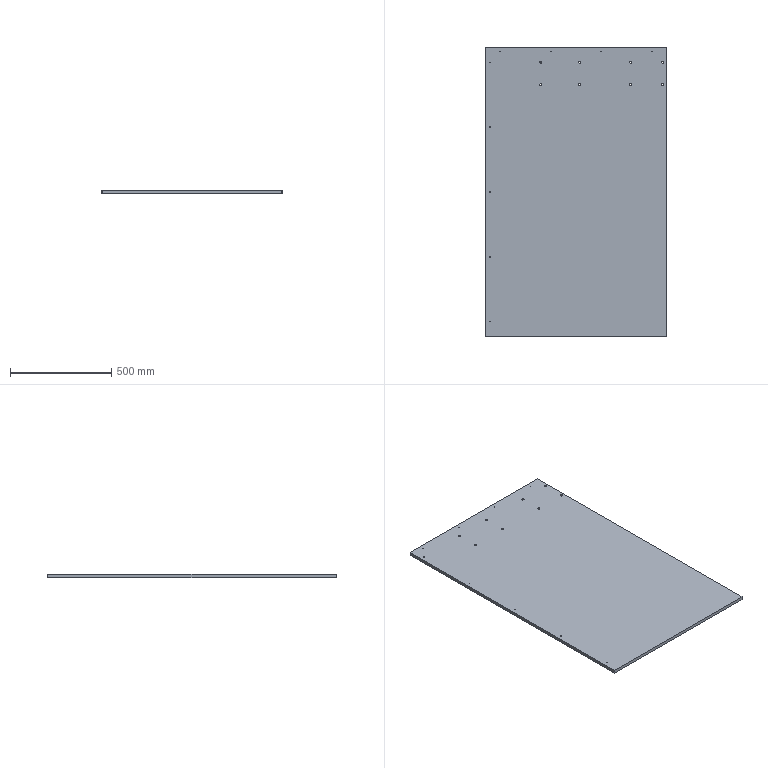Part | NX | features BREP 1 | 1 solid | 44 faces | box 895 x 1433 x 16 mm | volume 20507957 mm3 | cylinder 34 | plane 10 | commonest cylinder face diameters 3.3 x18 10.5 x16
STEP:
#1=CARTESIAN_POINT('',(-168.75,531.5,16.));
#2=VERTEX_POINT('',#1);
#3=CARTESIAN_POINT('',(-179.25,531.5,16.));
#4=VERTEX_POINT('',#3);
#5=CARTESIAN_POINT('',(-174.,531.5,16.));
#6=DIRECTION('',(0.,0.,-1.));
#7=DIRECTION('',(-1.,0.,0.));
#8=AXIS2_PLACEMENT_3D('',#5,#6,#7);
#9=CIRCLE('',#8,5.25);
#10=EDGE_CURVE('',#2,#4,#9,.T.);
#11=ORIENTED_EDGE('',*,*,#10,.F.);
#12=CARTESIAN_POINT('',(-168.75,531.5,0.));
#13=VERTEX_POINT('',#12);
#14=CARTESIAN_POINT('',(-168.75,531.5,0.));
#15=DIRECTION('',(0.,0.,-1.));
#16=VECTOR('',#15,1000.);
#17=LINE('',#14,#16);
#18=EDGE_CURVE('',#2,#13,#17,.T.);
#19=ORIENTED_EDGE('',*,*,#18,.T.);
#20=CARTESIAN_POINT('',(-179.25,531.5,0.));
#21=VERTEX_POINT('',#20);
#22=CARTESIAN_POINT('',(-174.,531.5,0.));
#23=DIRECTION('',(0.,0.,-1.));
#24=DIRECTION('',(-1.,0.,0.));
#25=AXIS2_PLACEMENT_3D('',#22,#23,#24);
#26=CIRCLE('',#25,5.25);
#27=EDGE_CURVE('',#13,#21,#26,.T.);
#28=ORIENTED_EDGE('',*,*,#27,.T.);
#29=CARTESIAN_POINT('',(-179.25,531.5,0.));
#30=DIRECTION('',(0.,0.,-1.));
#31=VECTOR('',#30,1000.);
#32=LINE('',#29,#31);
#33=EDGE_CURVE('',#4,#21,#32,.T.);
#34=ORIENTED_EDGE('',*,*,#33,.F.);
#35=EDGE_LOOP('',(#11,#19,#28,#34));
#36=FACE_BOUND('',#35,.T.);
#37=CARTESIAN_POINT('',(-174.,531.5,0.));
#38=DIRECTION('',(0.,0.,-1.));
#39=DIRECTION('',(-1.,0.,0.));
#40=AXIS2_PLACEMENT_3D('',#37,#38,#39);
#41=CYLINDRICAL_SURFACE('',#40,5.25);
#42=ADVANCED_FACE('',(#36),#41,.F.);
#43=CARTESIAN_POINT('',(-168.75,641.5,16.));
#44=VERTEX_POINT('',#43);
#45=CARTESIAN_POINT('',(-179.25,641.5,16.));
#46=VERTEX_POINT('',#45);
#47=CARTESIAN_POINT('',(-174.,641.5,16.));
#48=DIRECTION('',(0.,0.,-1.));
#49=DIRECTION('',(-1.,0.,0.));
#50=AXIS2_PLACEMENT_3D('',#47,#48,#49);
#51=CIRCLE('',#50,5.25);
#52=EDGE_CURVE('',#44,#46,#51,.T.);
#53=ORIENTED_EDGE('',*,*,#52,.F.);
#54=CARTESIAN_POINT('',(-168.75,641.5,0.));
#55=VERTEX_POINT('',#54);
#56=CARTESIAN_POINT('',(-168.75,641.5,0.));
#57=DIRECTION('',(0.,0.,-1.));
#58=VECTOR('',#57,1000.);
#59=LINE('',#56,#58);
#60=EDGE_CURVE('',#44,#55,#59,.T.);
#61=ORIENTED_EDGE('',*,*,#60,.T.);
#62=CARTESIAN_POINT('',(-179.25,641.5,0.));
#63=VERTEX_POINT('',#62);
#64=CARTESIAN_POINT('',(-174.,641.5,0.));
#65=DIRECTION('',(0.,0.,-1.));
#66=DIRECTION('',(-1.,0.,0.));
#67=AXIS2_PLACEMENT_3D('',#64,#65,#66);
#68=CIRCLE('',#67,5.25);
#69=EDGE_CURVE('',#55,#63,#68,.T.);
#70=ORIENTED_EDGE('',*,*,#69,.T.);
#71=CARTESIAN_POINT('',(-179.25,641.5,0.));
#72=DIRECTION('',(0.,0.,-1.));
#73=VECTOR('',#72,1000.);
#74=LINE('',#71,#73);
#75=EDGE_CURVE('',#46,#63,#74,.T.);
#76=ORIENTED_EDGE('',*,*,#75,.F.);
#77=EDGE_LOOP('',(#53,#61,#70,#76));
#78=FACE_BOUND('',#77,.T.);
#79=CARTESIAN_POINT('',(-174.,641.5,0.));
#80=DIRECTION('',(0.,0.,-1.));
#81=DIRECTION('',(-1.,0.,0.));
#82=AXIS2_PLACEMENT_3D('',#79,#80,#81);
#83=CYLINDRICAL_SURFACE('',#82,5.25);
#84=ADVANCED_FACE('',(#78),#83,.F.);
#85=CARTESIAN_POINT('',(23.75,531.5,16.));
#86=VERTEX_POINT('',#85);
#87=CARTESIAN_POINT('',(13.25,531.5,16.));
#88=VERTEX_POINT('',#87);
#89=CARTESIAN_POINT('',(18.5,531.5,16.));
#90=DIRECTION('',(0.,0.,-1.));
#91=DIRECTION('',(-1.,0.,0.));
#92=AXIS2_PLACEMENT_3D('',#89,#90,#91);
#93=CIRCLE('',#92,5.25);
#94=EDGE_CURVE('',#86,#88,#93,.T.);
#95=ORIENTED_EDGE('',*,*,#94,.F.);
#96=CARTESIAN_POINT('',(23.75,531.5,0.));
#97=VERTEX_POINT('',#96);
#98=CARTESIAN_POINT('',(23.75,531.5,0.));
#99=DIRECTION('',(0.,0.,-1.));
#100=VECTOR('',#99,1000.);
#101=LINE('',#98,#100);
#102=EDGE_CURVE('',#86,#97,#101,.T.);
#103=ORIENTED_EDGE('',*,*,#102,.T.);
#104=CARTESIAN_POINT('',(13.25,531.5,0.));
#105=VERTEX_POINT('',#104);
#106=CARTESIAN_POINT('',(18.5,531.5,0.));
#107=DIRECTION('',(0.,0.,-1.));
#108=DIRECTION('',(-1.,0.,0.));
#109=AXIS2_PLACEMENT_3D('',#106,#107,#108);
#110=CIRCLE('',#109,5.25);
#111=EDGE_CURVE('',#97,#105,#110,.T.);
#112=ORIENTED_EDGE('',*,*,#111,.T.);
#113=CARTESIAN_POINT('',(13.25,531.5,0.));
#114=DIRECTION('',(0.,0.,-1.));
#115=VECTOR('',#114,1000.);
#116=LINE('',#113,#115);
#117=EDGE_CURVE('',#88,#105,#116,.T.);
#118=ORIENTED_EDGE('',*,*,#117,.F.);
#119=EDGE_LOOP('',(#95,#103,#112,#118));
#120=FACE_BOUND('',#119,.T.);
#121=CARTESIAN_POINT('',(18.5,531.5,0.));
#122=DIRECTION('',(0.,0.,-1.));
#123=DIRECTION('',(-1.,0.,0.));
#124=AXIS2_PLACEMENT_3D('',#121,#122,#123);
#125=CYLINDRICAL_SURFACE('',#124,5.25);
#126=ADVANCED_FACE('',(#120),#125,.F.);
#127=CARTESIAN_POINT('',(23.75,641.5,16.));
#128=VERTEX_POINT('',#127);
#129=CARTESIAN_POINT('',(13.25,641.5,16.));
#130=VERTEX_POINT('',#129);
#131=CARTESIAN_POINT('',(18.5,641.5,16.));
#132=DIRECTION('',(0.,0.,-1.));
#133=DIRECTION('',(-1.,0.,0.));
#134=AXIS2_PLACEMENT_3D('',#131,#132,#133);
#135=CIRCLE('',#134,5.25);
#136=EDGE_CURVE('',#128,#130,#135,.T.);
#137=ORIENTED_EDGE('',*,*,#136,.F.);
#138=CARTESIAN_POINT('',(23.75,641.5,0.));
#139=VERTEX_POINT('',#138);
#140=CARTESIAN_POINT('',(23.75,641.5,0.));
#141=DIRECTION('',(0.,0.,-1.));
#142=VECTOR('',#141,1000.);
#143=LINE('',#140,#142);
#144=EDGE_CURVE('',#128,#139,#143,.T.);
#145=ORIENTED_EDGE('',*,*,#144,.T.);
#146=CARTESIAN_POINT('',(13.25,641.5,0.));
#147=VERTEX_POINT('',#146);
#148=CARTESIAN_POINT('',(18.5,641.5,0.));
#149=DIRECTION('',(0.,0.,-1.));
#150=DIRECTION('',(-1.,0.,0.));
#151=AXIS2_PLACEMENT_3D('',#148,#149,#150);
#152=CIRCLE('',#151,5.25);
#153=EDGE_CURVE('',#139,#147,#152,.T.);
#154=ORIENTED_EDGE('',*,*,#153,.T.);
#155=CARTESIAN_POINT('',(13.25,641.5,0.));
#156=DIRECTION('',(0.,0.,-1.));
#157=VECTOR('',#156,1000.);
#158=LINE('',#155,#157);
#159=EDGE_CURVE('',#130,#147,#158,.T.);
#160=ORIENTED_EDGE('',*,*,#159,.F.);
#161=EDGE_LOOP('',(#137,#145,#154,#160));
#162=FACE_BOUND('',#161,.T.);
#163=CARTESIAN_POINT('',(18.5,641.5,0.));
#164=DIRECTION('',(0.,0.,-1.));
#165=DIRECTION('',(-1.,0.,0.));
#166=AXIS2_PLACEMENT_3D('',#163,#164,#165);
#167=CYLINDRICAL_SURFACE('',#166,5.25);
#168=ADVANCED_FACE('',(#162),#167,.F.);
#169=CARTESIAN_POINT('',(275.75,531.5,16.));
#170=VERTEX_POINT('',#169);
#171=CARTESIAN_POINT('',(265.25,531.5,16.));
#172=VERTEX_POINT('',#171);
#173=CARTESIAN_POINT('',(270.5,531.5,16.));
#174=DIRECTION('',(0.,0.,-1.));
#175=DIRECTION('',(-1.,0.,0.));
#176=AXIS2_PLACEMENT_3D('',#173,#174,#175);
#177=CIRCLE('',#176,5.25);
#178=EDGE_CURVE('',#170,#172,#177,.T.);
#179=ORIENTED_EDGE('',*,*,#178,.F.);
#180=CARTESIAN_POINT('',(275.75,531.5,0.));
#181=VERTEX_POINT('',#180);
#182=CARTESIAN_POINT('',(275.75,531.5,0.));
#183=DIRECTION('',(0.,0.,-1.));
#184=VECTOR('',#183,1000.);
#185=LINE('',#182,#184);
#186=EDGE_CURVE('',#170,#181,#185,.T.);
#187=ORIENTED_EDGE('',*,*,#186,.T.);
#188=CARTESIAN_POINT('',(265.25,531.5,0.));
#189=VERTEX_POINT('',#188);
#190=CARTESIAN_POINT('',(270.5,531.5,0.));
#191=DIRECTION('',(0.,0.,-1.));
#192=DIRECTION('',(-1.,0.,0.));
#193=AXIS2_PLACEMENT_3D('',#190,#191,#192);
#194=CIRCLE('',#193,5.25);
#195=EDGE_CURVE('',#181,#189,#194,.T.);
#196=ORIENTED_EDGE('',*,*,#195,.T.);
#197=CARTESIAN_POINT('',(265.25,531.5,0.));
#198=DIRECTION('',(0.,0.,-1.));
#199=VECTOR('',#198,1000.);
#200=LINE('',#197,#199);
#201=EDGE_CURVE('',#172,#189,#200,.T.);
#202=ORIENTED_EDGE('',*,*,#201,.F.);
#203=EDGE_LOOP('',(#179,#187,#196,#202));
#204=FACE_BOUND('',#203,.T.);
#205=CARTESIAN_POINT('',(270.5,531.5,0.));
#206=DIRECTION('',(0.,0.,-1.));
#207=DIRECTION('',(-1.,0.,0.));
#208=AXIS2_PLACEMENT_3D('',#205,#206,#207);
#209=CYLINDRICAL_SURFACE('',#208,5.25);
#210=ADVANCED_FACE('',(#204),#209,.F.);
#211=CARTESIAN_POINT('',(275.75,641.5,16.));
#212=VERTEX_POINT('',#211);
#213=CARTESIAN_POINT('',(265.25,641.5,16.));
#214=VERTEX_POINT('',#213);
#215=CARTESIAN_POINT('',(270.5,641.5,16.));
#216=DIRECTION('',(0.,0.,-1.));
#217=DIRECTION('',(-1.,0.,0.));
#218=AXIS2_PLACEMENT_3D('',#215,#216,#217);
#219=CIRCLE('',#218,5.25);
#220=EDGE_CURVE('',#212,#214,#219,.T.);
#221=ORIENTED_EDGE('',*,*,#220,.F.);
#222=CARTESIAN_POINT('',(275.75,641.5,0.));
#223=VERTEX_POINT('',#222);
#224=CARTESIAN_POINT('',(275.75,641.5,0.));
#225=DIRECTION('',(0.,0.,-1.));
#226=VECTOR('',#225,1000.);
#227=LINE('',#224,#226);
#228=EDGE_CURVE('',#212,#223,#227,.T.);
#229=ORIENTED_EDGE('',*,*,#228,.T.);
#230=CARTESIAN_POINT('',(265.25,641.5,0.));
#231=VERTEX_POINT('',#230);
#232=CARTESIAN_POINT('',(270.5,641.5,0.));
#233=DIRECTION('',(0.,0.,-1.));
#234=DIRECTION('',(-1.,0.,0.));
#235=AXIS2_PLACEMENT_3D('',#232,#233,#234);
#236=CIRCLE('',#235,5.25);
#237=EDGE_CURVE('',#223,#231,#236,.T.);
#238=ORIENTED_EDGE('',*,*,#237,.T.);
#239=CARTESIAN_POINT('',(265.25,641.5,0.));
#240=DIRECTION('',(0.,0.,-1.));
#241=VECTOR('',#240,1000.);
#242=LINE('',#239,#241);
#243=EDGE_CURVE('',#214,#231,#242,.T.);
#244=ORIENTED_EDGE('',*,*,#243,.F.);
#245=EDGE_LOOP('',(#221,#229,#238,#244));
#246=FACE_BOUND('',#245,.T.);
#247=CARTESIAN_POINT('',(270.5,641.5,0.));
#248=DIRECTION('',(0.,0.,-1.));
#249=DIRECTION('',(-1.,0.,0.));
#250=AXIS2_PLACEMENT_3D('',#247,#248,#249);
#251=CYLINDRICAL_SURFACE('',#250,5.25);
#252=ADVANCED_FACE('',(#246),#251,.F.);
#253=CARTESIAN_POINT('',(434.25,641.5,16.));
#254=VERTEX_POINT('',#253);
#255=CARTESIAN_POINT('',(423.75,641.5,16.));
#256=VERTEX_POINT('',#255);
#257=CARTESIAN_POINT('',(429.,641.5,16.));
#258=DIRECTION('',(0.,0.,-1.));
#259=DIRECTION('',(-1.,0.,0.));
#260=AXIS2_PLACEMENT_3D('',#257,#258,#259);
#261=CIRCLE('',#260,5.25);
#262=EDGE_CURVE('',#254,#256,#261,.T.);
#263=ORIENTED_EDGE('',*,*,#262,.F.);
#264=CARTESIAN_POINT('',(434.25,641.5,0.));
#265=VERTEX_POINT('',#264);
#266=CARTESIAN_POINT('',(434.25,641.5,0.));
#267=DIRECTION('',(0.,0.,-1.));
#268=VECTOR('',#267,1000.);
#269=LINE('',#266,#268);
#270=EDGE_CURVE('',#254,#265,#269,.T.);
#271=ORIENTED_EDGE('',*,*,#270,.T.);
#272=CARTESIAN_POINT('',(423.75,641.5,0.));
#273=VERTEX_POINT('',#272);
#274=CARTESIAN_POINT('',(429.,641.5,0.));
#275=DIRECTION('',(0.,0.,-1.));
#276=DIRECTION('',(-1.,0.,0.));
#277=AXIS2_PLACEMENT_3D('',#274,#275,#276);
#278=CIRCLE('',#277,5.25);
#279=EDGE_CURVE('',#265,#273,#278,.T.);
#280=ORIENTED_EDGE('',*,*,#279,.T.);
#281=CARTESIAN_POINT('',(423.75,641.5,0.));
#282=DIRECTION('',(0.,0.,-1.));
#283=VECTOR('',#282,1000.);
#284=LINE('',#281,#283);
#285=EDGE_CURVE('',#256,#273,#284,.T.);
#286=ORIENTED_EDGE('',*,*,#285,.F.);
#287=EDGE_LOOP('',(#263,#271,#280,#286));
#288=FACE_BOUND('',#287,.T.);
#289=CARTESIAN_POINT('',(429.,641.5,0.));
#290=DIRECTION('',(0.,0.,-1.));
#291=DIRECTION('',(-1.,0.,0.));
#292=AXIS2_PLACEMENT_3D('',#289,#290,#291);
#293=CYLINDRICAL_SURFACE('',#292,5.25);
#294=ADVANCED_FACE('',(#288),#293,.F.);
#295=CARTESIAN_POINT('',(434.25,531.5,16.));
#296=VERTEX_POINT('',#295);
#297=CARTESIAN_POINT('',(423.75,531.5,16.));
#298=VERTEX_POINT('',#297);
#299=CARTESIAN_POINT('',(429.,531.5,16.));
#300=DIRECTION('',(0.,0.,-1.));
#301=DIRECTION('',(-1.,0.,0.));
#302=AXIS2_PLACEMENT_3D('',#299,#300,#301);
#303=CIRCLE('',#302,5.25);
#304=EDGE_CURVE('',#296,#298,#303,.T.);
#305=ORIENTED_EDGE('',*,*,#304,.F.);
#306=CARTESIAN_POINT('',(434.25,531.5,0.));
#307=VERTEX_POINT('',#306);
#308=CARTESIAN_POINT('',(434.25,531.5,0.));
#309=DIRECTION('',(0.,0.,-1.));
#310=VECTOR('',#309,1000.);
#311=LINE('',#308,#310);
#312=EDGE_CURVE('',#296,#307,#311,.T.);
#313=ORIENTED_EDGE('',*,*,#312,.T.);
#314=CARTESIAN_POINT('',(423.75,531.5,0.));
#315=VERTEX_POINT('',#314);
#316=CARTESIAN_POINT('',(429.,531.5,0.));
#317=DIRECTION('',(0.,0.,-1.));
#318=DIRECTION('',(-1.,0.,0.));
#319=AXIS2_PLACEMENT_3D('',#316,#317,#318);
#320=CIRCLE('',#319,5.25);
#321=EDGE_CURVE('',#307,#315,#320,.T.);
#322=ORIENTED_EDGE('',*,*,#321,.T.);
#323=CARTESIAN_POINT('',(423.75,531.5,0.));
#324=DIRECTION('',(0.,0.,-1.));
#325=VECTOR('',#324,1000.);
#326=LINE('',#323,#325);
#327=EDGE_CURVE('',#298,#315,#326,.T.);
#328=ORIENTED_EDGE('',*,*,#327,.F.);
#329=EDGE_LOOP('',(#305,#313,#322,#328));
#330=FACE_BOUND('',#329,.T.);
#331=CARTESIAN_POINT('',(429.,531.5,0.));
#332=DIRECTION('',(0.,0.,-1.));
#333=DIRECTION('',(-1.,0.,0.));
#334=AXIS2_PLACEMENT_3D('',#331,#332,#333);
#335=CYLINDRICAL_SURFACE('',#334,5.25);
#336=ADVANCED_FACE('',(#330),#335,.F.);
#337=CARTESIAN_POINT('',(-423.35,-640.,16.));
#338=VERTEX_POINT('',#337);
#339=CARTESIAN_POINT('',(-426.65,-640.,16.));
#340=VERTEX_POINT('',#339);
#341=CARTESIAN_POINT('',(-425.,-640.,16.));
#342=DIRECTION('',(0.,0.,-1.));
#343=DIRECTION('',(-1.,0.,0.));
#344=AXIS2_PLACEMENT_3D('',#341,#342,#343);
#345=CIRCLE('',#344,1.65);
#346=EDGE_CURVE('',#338,#340,#345,.T.);
#347=ORIENTED_EDGE('',*,*,#346,.F.);
#348=CARTESIAN_POINT('',(-423.35,-640.,0.));
#349=VERTEX_POINT('',#348);
#350=CARTESIAN_POINT('',(-423.35,-640.,0.));
#351=DIRECTION('',(0.,0.,-1.));
#352=VECTOR('',#351,1000.);
#353=LINE('',#350,#352);
#354=EDGE_CURVE('',#338,#349,#353,.T.);
#355=ORIENTED_EDGE('',*,*,#354,.T.);
#356=CARTESIAN_POINT('',(-426.65,-640.,0.));
#357=VERTEX_POINT('',#356);
#358=CARTESIAN_POINT('',(-425.,-640.,0.));
#359=DIRECTION('',(0.,0.,-1.));
#360=DIRECTION('',(-1.,0.,0.));
#361=AXIS2_PLACEMENT_3D('',#358,#359,#360);
#362=CIRCLE('',#361,1.65);
#363=EDGE_CURVE('',#349,#357,#362,.T.);
#364=ORIENTED_EDGE('',*,*,#363,.T.);
#365=CARTESIAN_POINT('',(-426.65,-640.,0.));
#366=DIRECTION('',(0.,0.,-1.));
#367=VECTOR('',#366,1000.);
#368=LINE('',#365,#367);
#369=EDGE_CURVE('',#340,#357,#368,.T.);
#370=ORIENTED_EDGE('',*,*,#369,.F.);
#371=EDGE_LOOP('',(#347,#355,#364,#370));
#372=FACE_BOUND('',#371,.T.);
#373=CARTESIAN_POINT('',(-425.,-640.,0.));
#374=DIRECTION('',(0.,0.,-1.));
#375=DIRECTION('',(-1.,0.,0.));
#376=AXIS2_PLACEMENT_3D('',#373,#374,#375);
#377=CYLINDRICAL_SURFACE('',#376,1.65);
#378=ADVANCED_FACE('',(#372),#377,.F.);
#379=CARTESIAN_POINT('',(-423.35,0.,16.));
#380=VERTEX_POINT('',#379);
#381=CARTESIAN_POINT('',(-426.65,0.,16.));
#382=VERTEX_POINT('',#381);
#383=CARTESIAN_POINT('',(-425.,0.,16.));
#384=DIRECTION('',(0.,0.,-1.));
#385=DIRECTION('',(-1.,0.,0.));
#386=AXIS2_PLACEMENT_3D('',#383,#384,#385);
#387=CIRCLE('',#386,1.65);
#388=EDGE_CURVE('',#380,#382,#387,.T.);
#389=ORIENTED_EDGE('',*,*,#388,.F.);
#390=CARTESIAN_POINT('',(-423.35,0.,0.));
#391=VERTEX_POINT('',#390);
#392=CARTESIAN_POINT('',(-423.35,0.,0.));
#393=DIRECTION('',(0.,0.,-1.));
#394=VECTOR('',#393,1000.);
#395=LINE('',#392,#394);
#396=EDGE_CURVE('',#380,#391,#395,.T.);
#397=ORIENTED_EDGE('',*,*,#396,.T.);
#398=CARTESIAN_POINT('',(-426.65,0.,0.));
#399=VERTEX_POINT('',#398);
#400=CARTESIAN_POINT('',(-425.,0.,0.));
#401=DIRECTION('',(0.,0.,-1.));
#402=DIRECTION('',(-1.,0.,0.));
#403=AXIS2_PLACEMENT_3D('',#400,#401,#402);
#404=CIRCLE('',#403,1.65);
#405=EDGE_CURVE('',#391,#399,#404,.T.);
#406=ORIENTED_EDGE('',*,*,#405,.T.);
#407=CARTESIAN_POINT('',(-426.65,0.,0.));
#408=DIRECTION('',(0.,0.,-1.));
#409=VECTOR('',#408,1000.);
#410=LINE('',#407,#409);
#411=EDGE_CURVE('',#382,#399,#410,.T.);
#412=ORIENTED_EDGE('',*,*,#411,.F.);
#413=EDGE_LOOP('',(#389,#397,#406,#412));
#414=FACE_BOUND('',#413,.T.);
#415=CARTESIAN_POINT('',(-425.,0.,0.));
#416=DIRECTION('',(0.,0.,-1.));
#417=DIRECTION('',(-1.,0.,0.));
#418=AXIS2_PLACEMENT_3D('',#415,#416,#417);
#419=CYLINDRICAL_SURFACE('',#418,1.65);
#420=ADVANCED_FACE('',(#414),#419,.F.);
#421=CARTESIAN_POINT('',(-423.35,320.,16.));
#422=VERTEX_POINT('',#421);
#423=CARTESIAN_POINT('',(-426.65,320.,16.));
#424=VERTEX_POINT('',#423);
#425=CARTESIAN_POINT('',(-425.,320.,16.));
#426=DIRECTION('',(0.,0.,-1.));
#427=DIRECTION('',(-1.,0.,0.));
#428=AXIS2_PLACEMENT_3D('',#425,#426,#427);
#429=CIRCLE('',#428,1.65);
#430=EDGE_CURVE('',#422,#424,#429,.T.);
#431=ORIENTED_EDGE('',*,*,#430,.F.);
#432=CARTESIAN_POINT('',(-423.35,320.,0.));
#433=VERTEX_POINT('',#432);
#434=CARTESIAN_POINT('',(-423.35,320.,0.));
#435=DIRECTION('',(0.,0.,-1.));
#436=VECTOR('',#435,1000.);
#437=LINE('',#434,#436);
#438=EDGE_CURVE('',#422,#433,#437,.T.);
#439=ORIENTED_EDGE('',*,*,#438,.T.);
#440=CARTESIAN_POINT('',(-426.65,320.,0.));
#441=VERTEX_POINT('',#440);
#442=CARTESIAN_POINT('',(-425.,320.,0.));
#443=DIRECTION('',(0.,0.,-1.));
#444=DIRECTION('',(-1.,0.,0.));
#445=AXIS2_PLACEMENT_3D('',#442,#443,#444);
#446=CIRCLE('',#445,1.65);
#447=EDGE_CURVE('',#433,#441,#446,.T.);
#448=ORIENTED_EDGE('',*,*,#447,.T.);
#449=CARTESIAN_POINT('',(-426.65,320.,0.));
#450=DIRECTION('',(0.,0.,-1.));
#451=VECTOR('',#450,1000.);
#452=LINE('',#449,#451);
#453=EDGE_CURVE('',#424,#441,#452,.T.);
#454=ORIENTED_EDGE('',*,*,#453,.F.);
#455=EDGE_LOOP('',(#431,#439,#448,#454));
#456=FACE_BOUND('',#455,.T.);
#457=CARTESIAN_POINT('',(-425.,320.,0.));
#458=DIRECTION('',(0.,0.,-1.));
#459=DIRECTION('',(-1.,0.,0.));
#460=AXIS2_PLACEMENT_3D('',#457,#458,#459);
#461=CYLINDRICAL_SURFACE('',#460,1.65);
#462=ADVANCED_FACE('',(#456),#461,.F.);
#463=CARTESIAN_POINT('',(-123.35,694.,16.));
#464=VERTEX_POINT('',#463);
#465=CARTESIAN_POINT('',(-126.65,694.,16.));
#466=VERTEX_POINT('',#465);
#467=CARTESIAN_POINT('',(-125.,694.,16.));
#468=DIRECTION('',(0.,0.,-1.));
#469=DIRECTION('',(-1.,0.,0.));
#470=AXIS2_PLACEMENT_3D('',#467,#468,#469);
#471=CIRCLE('',#470,1.65);
#472=EDGE_CURVE('',#464,#466,#471,.T.);
#473=ORIENTED_EDGE('',*,*,#472,.F.);
#474=CARTESIAN_POINT('',(-123.35,694.,0.));
#475=VERTEX_POINT('',#474);
#476=CARTESIAN_POINT('',(-123.35,694.,0.));
#477=DIRECTION('',(0.,0.,-1.));
#478=VECTOR('',#477,1000.);
#479=LINE('',#476,#478);
#480=EDGE_CURVE('',#464,#475,#479,.T.);
#481=ORIENTED_EDGE('',*,*,#480,.T.);
#482=CARTESIAN_POINT('',(-126.65,694.,0.));
#483=VERTEX_POINT('',#482);
#484=CARTESIAN_POINT('',(-125.,694.,0.));
#485=DIRECTION('',(0.,0.,-1.));
#486=DIRECTION('',(-1.,0.,0.));
#487=AXIS2_PLACEMENT_3D('',#484,#485,#486);
#488=CIRCLE('',#487,1.65);
#489=EDGE_CURVE('',#475,#483,#488,.T.);
#490=ORIENTED_EDGE('',*,*,#489,.T.);
#491=CARTESIAN_POINT('',(-126.65,694.,0.));
#492=DIRECTION('',(0.,0.,-1.));
#493=VECTOR('',#492,1000.);
#494=LINE('',#491,#493);
#495=EDGE_CURVE('',#466,#483,#494,.T.);
#496=ORIENTED_EDGE('',*,*,#495,.F.);
#497=EDGE_LOOP('',(#473,#481,#490,#496));
#498=FACE_BOUND('',#497,.T.);
#499=CARTESIAN_POINT('',(-125.,694.,0.));
#500=DIRECTION('',(0.,0.,-1.));
#501=DIRECTION('',(-1.,0.,0.));
#502=AXIS2_PLACEMENT_3D('',#499,#500,#501);
#503=CYLINDRICAL_SURFACE('',#502,1.65);
#504=ADVANCED_FACE('',(#498),#503,.F.);
#505=CARTESIAN_POINT('',(-423.35,-320.,16.));
#506=VERTEX_POINT('',#505);
#507=CARTESIAN_POINT('',(-426.65,-320.,16.));
#508=VERTEX_POINT('',#507);
#509=CARTESIAN_POINT('',(-425.,-320.,16.));
#510=DIRECTION('',(0.,0.,-1.));
#511=DIRECTION('',(-1.,0.,0.));
#512=AXIS2_PLACEMENT_3D('',#509,#510,#511);
#513=CIRCLE('',#512,1.65);
#514=EDGE_CURVE('',#506,#508,#513,.T.);
#515=ORIENTED_EDGE('',*,*,#514,.F.);
#516=CARTESIAN_POINT('',(-423.35,-320.,0.));
#517=VERTEX_POINT('',#516);
#518=CARTESIAN_POINT('',(-423.35,-320.,0.));
#519=DIRECTION('',(0.,0.,-1.));
#520=VECTOR('',#519,1000.);
#521=LINE('',#518,#520);
#522=EDGE_CURVE('',#506,#517,#521,.T.);
#523=ORIENTED_EDGE('',*,*,#522,.T.);
#524=CARTESIAN_POINT('',(-426.65,-320.,0.));
#525=VERTEX_POINT('',#524);
#526=CARTESIAN_POINT('',(-425.,-320.,0.));
#527=DIRECTION('',(0.,0.,-1.));
#528=DIRECTION('',(-1.,0.,0.));
#529=AXIS2_PLACEMENT_3D('',#526,#527,#528);
#530=CIRCLE('',#529,1.65);
#531=EDGE_CURVE('',#517,#525,#530,.T.);
#532=ORIENTED_EDGE('',*,*,#531,.T.);
#533=CARTESIAN_POINT('',(-426.65,-320.,0.));
#534=DIRECTION('',(0.,0.,-1.));
#535=VECTOR('',#534,1000.);
#536=LINE('',#533,#535);
#537=EDGE_CURVE('',#508,#525,#536,.T.);
#538=ORIENTED_EDGE('',*,*,#537,.F.);
#539=EDGE_LOOP('',(#515,#523,#532,#538));
#540=FACE_BOUND('',#539,.T.);
#541=CARTESIAN_POINT('',(-425.,-320.,0.));
#542=DIRECTION('',(0.,0.,-1.));
#543=DIRECTION('',(-1.,0.,0.));
#544=AXIS2_PLACEMENT_3D('',#541,#542,#543);
#545=CYLINDRICAL_SURFACE('',#544,1.65);
#546=ADVANCED_FACE('',(#540),#545,.F.);
#547=CARTESIAN_POINT('',(-373.35,694.,16.));
#548=VERTEX_POINT('',#547);
#549=CARTESIAN_POINT('',(-376.65,694.,16.));
#550=VERTEX_POINT('',#549);
#551=CARTESIAN_POINT('',(-375.,694.,16.));
#552=DIRECTION('',(0.,0.,-1.));
#553=DIRECTION('',(-1.,0.,0.));
#554=AXIS2_PLACEMENT_3D('',#551,#552,#553);
#555=CIRCLE('',#554,1.65);
#556=EDGE_CURVE('',#548,#550,#555,.T.);
#557=ORIENTED_EDGE('',*,*,#556,.F.);
#558=CARTESIAN_POINT('',(-373.35,694.,0.));
#559=VERTEX_POINT('',#558);
#560=CARTESIAN_POINT('',(-373.35,694.,0.));
#561=DIRECTION('',(0.,0.,-1.));
#562=VECTOR('',#561,1000.);
#563=LINE('',#560,#562);
#564=EDGE_CURVE('',#548,#559,#563,.T.);
#565=ORIENTED_EDGE('',*,*,#564,.T.);
#566=CARTESIAN_POINT('',(-376.65,694.,0.));
#567=VERTEX_POINT('',#566);
#568=CARTESIAN_POINT('',(-375.,694.,0.));
#569=DIRECTION('',(0.,0.,-1.));
#570=DIRECTION('',(-1.,0.,0.));
#571=AXIS2_PLACEMENT_3D('',#568,#569,#570);
#572=CIRCLE('',#571,1.65);
#573=EDGE_CURVE('',#559,#567,#572,.T.);
#574=ORIENTED_EDGE('',*,*,#573,.T.);
#575=CARTESIAN_POINT('',(-376.65,694.,0.));
#576=DIRECTION('',(0.,0.,-1.));
#577=VECTOR('',#576,1000.);
#578=LINE('',#575,#577);
#579=EDGE_CURVE('',#550,#567,#578,.T.);
#580=ORIENTED_EDGE('',*,*,#579,.F.);
#581=EDGE_LOOP('',(#557,#565,#574,#580));
#582=FACE_BOUND('',#581,.T.);
#583=CARTESIAN_POINT('',(-375.,694.,0.));
#584=DIRECTION('',(0.,0.,-1.));
#585=DIRECTION('',(-1.,0.,0.));
#586=AXIS2_PLACEMENT_3D('',#583,#584,#585);
#587=CYLINDRICAL_SURFACE('',#586,1.65);
#588=ADVANCED_FACE('',(#582),#587,.F.);
#589=CARTESIAN_POINT('',(-423.35,640.,16.));
#590=VERTEX_POINT('',#589);
#591=CARTESIAN_POINT('',(-426.65,640.,16.));
#592=VERTEX_POINT('',#591);
#593=CARTESIAN_POINT('',(-425.,640.,16.));
#594=DIRECTION('',(0.,0.,-1.));
#595=DIRECTION('',(-1.,0.,0.));
#596=AXIS2_PLACEMENT_3D('',#593,#594,#595);
#597=CIRCLE('',#596,1.65);
#598=EDGE_CURVE('',#590,#592,#597,.T.);
#599=ORIENTED_EDGE('',*,*,#598,.F.);
#600=CARTESIAN_POINT('',(-423.35,640.,0.));
#601=VERTEX_POINT('',#600);
#602=CARTESIAN_POINT('',(-423.35,640.,0.));
#603=DIRECTION('',(0.,0.,-1.));
#604=VECTOR('',#603,1000.);
#605=LINE('',#602,#604);
#606=EDGE_CURVE('',#590,#601,#605,.T.);
#607=ORIENTED_EDGE('',*,*,#606,.T.);
#608=CARTESIAN_POINT('',(-426.65,640.,0.));
#609=VERTEX_POINT('',#608);
#610=CARTESIAN_POINT('',(-425.,640.,0.));
#611=DIRECTION('',(0.,0.,-1.));
#612=DIRECTION('',(-1.,0.,0.));
#613=AXIS2_PLACEMENT_3D('',#610,#611,#612);
#614=CIRCLE('',#613,1.65);
#615=EDGE_CURVE('',#601,#609,#614,.T.);
#616=ORIENTED_EDGE('',*,*,#615,.T.);
#617=CARTESIAN_POINT('',(-426.65,640.,0.));
#618=DIRECTION('',(0.,0.,-1.));
#619=VECTOR('',#618,1000.);
#620=LINE('',#617,#619);
#621=EDGE_CURVE('',#592,#609,#620,.T.);
#622=ORIENTED_EDGE('',*,*,#621,.F.);
#623=EDGE_LOOP('',(#599,#607,#616,#622));
#624=FACE_BOUND('',#623,.T.);
#625=CARTESIAN_POINT('',(-425.,640.,0.));
#626=DIRECTION('',(0.,0.,-1.));
#627=DIRECTION('',(-1.,0.,0.));
#628=AXIS2_PLACEMENT_3D('',#625,#626,#627);
#629=CYLINDRICAL_SURFACE('',#628,1.65);
#630=ADVANCED_FACE('',(#624),#629,.F.);
#631=CARTESIAN_POINT('',(376.65,694.,16.));
#632=VERTEX_POINT('',#631);
#633=CARTESIAN_POINT('',(373.35,694.,16.));
#634=VERTEX_POINT('',#633);
#635=CARTESIAN_POINT('',(375.,694.,16.));
#636=DIRECTION('',(0.,0.,-1.));
#637=DIRECTION('',(-1.,0.,0.));
#638=AXIS2_PLACEMENT_3D('',#635,#636,#637);
#639=CIRCLE('',#638,1.65);
#640=EDGE_CURVE('',#632,#634,#639,.T.);
#641=ORIENTED_EDGE('',*,*,#640,.F.);
#642=CARTESIAN_POINT('',(376.65,694.,0.));
#643=VERTEX_POINT('',#642);
#644=CARTESIAN_POINT('',(376.65,694.,0.));
#645=DIRECTION('',(0.,0.,-1.));
#646=VECTOR('',#645,1000.);
#647=LINE('',#644,#646);
#648=EDGE_CURVE('',#632,#643,#647,.T.);
#649=ORIENTED_EDGE('',*,*,#648,.T.);
#650=CARTESIAN_POINT('',(373.35,694.,0.));
#651=VERTEX_POINT('',#650);
#652=CARTESIAN_POINT('',(375.,694.,0.));
#653=DIRECTION('',(0.,0.,-1.));
#654=DIRECTION('',(-1.,0.,0.));
#655=AXIS2_PLACEMENT_3D('',#652,#653,#654);
#656=CIRCLE('',#655,1.65);
#657=EDGE_CURVE('',#643,#651,#656,.T.);
#658=ORIENTED_EDGE('',*,*,#657,.T.);
#659=CARTESIAN_POINT('',(373.35,694.,0.));
#660=DIRECTION('',(0.,0.,-1.));
#661=VECTOR('',#660,1000.);
#662=LINE('',#659,#661);
#663=EDGE_CURVE('',#634,#651,#662,.T.);
#664=ORIENTED_EDGE('',*,*,#663,.F.);
#665=EDGE_LOOP('',(#641,#649,#658,#664));
#666=FACE_BOUND('',#665,.T.);
#667=CARTESIAN_POINT('',(375.,694.,0.));
#668=DIRECTION('',(0.,0.,-1.));
#669=DIRECTION('',(-1.,0.,0.));
#670=AXIS2_PLACEMENT_3D('',#667,#668,#669);
#671=CYLINDRICAL_SURFACE('',#670,1.65);
#672=ADVANCED_FACE('',(#666),#671,.F.);
#673=CARTESIAN_POINT('',(126.65,694.,16.));
#674=VERTEX_POINT('',#673);
#675=CARTESIAN_POINT('',(123.35,694.,16.));
#676=VERTEX_POINT('',#675);
#677=CARTESIAN_POINT('',(125.,694.,16.));
#678=DIRECTION('',(0.,0.,-1.));
#679=DIRECTION('',(-1.,0.,0.));
#680=AXIS2_PLACEMENT_3D('',#677,#678,#679);
#681=CIRCLE('',#680,1.65);
#682=EDGE_CURVE('',#674,#676,#681,.T.);
#683=ORIENTED_EDGE('',*,*,#682,.F.);
#684=CARTESIAN_POINT('',(126.65,694.,0.));
#685=VERTEX_POINT('',#684);
#686=CARTESIAN_POINT('',(126.65,694.,0.));
#687=DIRECTION('',(0.,0.,-1.));
#688=VECTOR('',#687,1000.);
#689=LINE('',#686,#688);
#690=EDGE_CURVE('',#674,#685,#689,.T.);
#691=ORIENTED_EDGE('',*,*,#690,.T.);
#692=CARTESIAN_POINT('',(123.35,694.,0.));
#693=VERTEX_POINT('',#692);
#694=CARTESIAN_POINT('',(125.,694.,0.));
#695=DIRECTION('',(0.,0.,-1.));
#696=DIRECTION('',(-1.,0.,0.));
#697=AXIS2_PLACEMENT_3D('',#694,#695,#696);
#698=CIRCLE('',#697,1.65);
#699=EDGE_CURVE('',#685,#693,#698,.T.);
#700=ORIENTED_EDGE('',*,*,#699,.T.);
#701=CARTESIAN_POINT('',(123.35,694.,0.));
#702=DIRECTION('',(0.,0.,-1.));
#703=VECTOR('',#702,1000.);
#704=LINE('',#701,#703);
#705=EDGE_CURVE('',#676,#693,#704,.T.);
#706=ORIENTED_EDGE('',*,*,#705,.F.);
#707=EDGE_LOOP('',(#683,#691,#700,#706));
#708=FACE_BOUND('',#707,.T.);
#709=CARTESIAN_POINT('',(125.,694.,0.));
#710=DIRECTION('',(0.,0.,-1.));
#711=DIRECTION('',(-1.,0.,0.));
#712=AXIS2_PLACEMENT_3D('',#709,#710,#711);
#713=CYLINDRICAL_SURFACE('',#712,1.65);
#714=ADVANCED_FACE('',(#708),#713,.F.);
#715=CARTESIAN_POINT('',(447.5,-713.5,16.));
#716=VERTEX_POINT('',#715);
#717=CARTESIAN_POINT('',(447.5,713.5,16.));
#718=VERTEX_POINT('',#717);
#719=CARTESIAN_POINT('',(447.5,716.5,16.));
#720=DIRECTION('',(0.,1.,0.));
#721=VECTOR('',#720,1000.);
#722=LINE('',#719,#721);
#723=EDGE_CURVE('',#716,#718,#722,.T.);
#724=ORIENTED_EDGE('',*,*,#723,.F.);
#725=CARTESIAN_POINT('',(447.5,-713.5,0.));
#726=VERTEX_POINT('',#725);
#727=CARTESIAN_POINT('',(447.5,-713.5,16.));
#728=DIRECTION('',(0.,0.,-1.));
#729=VECTOR('',#728,1000.);
#730=LINE('',#727,#729);
#731=EDGE_CURVE('',#716,#726,#730,.T.);
#732=ORIENTED_EDGE('',*,*,#731,.T.);
#733=CARTESIAN_POINT('',(447.5,713.5,0.));
#734=VERTEX_POINT('',#733);
#735=CARTESIAN_POINT('',(447.5,716.5,0.));
#736=DIRECTION('',(0.,1.,0.));
#737=VECTOR('',#736,1000.);
#738=LINE('',#735,#737);
#739=EDGE_CURVE('',#726,#734,#738,.T.);
#740=ORIENTED_EDGE('',*,*,#739,.T.);
#741=CARTESIAN_POINT('',(447.5,713.5,16.));
#742=DIRECTION('',(0.,0.,1.));
#743=VECTOR('',#742,1000.);
#744=LINE('',#741,#743);
#745=EDGE_CURVE('',#734,#718,#744,.T.);
#746=ORIENTED_EDGE('',*,*,#745,.T.);
#747=EDGE_LOOP('',(#724,#732,#740,#746));
#748=FACE_BOUND('',#747,.T.);
#749=CARTESIAN_POINT('',(447.5,716.5,16.));
#750=DIRECTION('',(-1.,0.,0.));
#751=DIRECTION('',(0.,1.,0.));
#752=AXIS2_PLACEMENT_3D('',#749,#750,#751);
#753=PLANE('',#752);
#754=ADVANCED_FACE('',(#748),#753,.F.);
#755=CARTESIAN_POINT('',(444.5,716.5,0.));
#756=VERTEX_POINT('',#755);
#757=CARTESIAN_POINT('',(-444.5,716.5,0.));
#758=VERTEX_POINT('',#757);
#759=CARTESIAN_POINT('',(-447.5,716.5,0.));
#760=DIRECTION('',(-1.,0.,0.));
#761=VECTOR('',#760,1000.);
#762=LINE('',#759,#761);
#763=EDGE_CURVE('',#756,#758,#762,.T.);
#764=ORIENTED_EDGE('',*,*,#763,.T.);
#765=CARTESIAN_POINT('',(-444.5,716.5,16.));
#766=VERTEX_POINT('',#765);
#767=CARTESIAN_POINT('',(-444.5,716.5,16.));
#768=DIRECTION('',(0.,0.,1.));
#769=VECTOR('',#768,1000.);
#770=LINE('',#767,#769);
#771=EDGE_CURVE('',#758,#766,#770,.T.);
#772=ORIENTED_EDGE('',*,*,#771,.T.);
#773=CARTESIAN_POINT('',(444.5,716.5,16.));
#774=VERTEX_POINT('',#773);
#775=CARTESIAN_POINT('',(-447.5,716.5,16.));
#776=DIRECTION('',(-1.,0.,0.));
#777=VECTOR('',#776,1000.);
#778=LINE('',#775,#777);
#779=EDGE_CURVE('',#774,#766,#778,.T.);
#780=ORIENTED_EDGE('',*,*,#779,.F.);
#781=CARTESIAN_POINT('',(444.5,716.5,16.));
#782=DIRECTION('',(0.,0.,-1.));
#783=VECTOR('',#782,1000.);
#784=LINE('',#781,#783);
#785=EDGE_CURVE('',#774,#756,#784,.T.);
#786=ORIENTED_EDGE('',*,*,#785,.T.);
#787=EDGE_LOOP('',(#764,#772,#780,#786));
#788=FACE_BOUND('',#787,.T.);
#789=CARTESIAN_POINT('',(-447.5,716.5,16.));
#790=DIRECTION('',(0.,-1.,0.));
#791=DIRECTION('',(0.,0.,-1.));
#792=AXIS2_PLACEMENT_3D('',#789,#790,#791);
#793=PLANE('',#792);
#794=ADVANCED_FACE('',(#788),#793,.F.);
#795=CARTESIAN_POINT('',(-447.5,713.5,0.));
#796=VERTEX_POINT('',#795);
#797=CARTESIAN_POINT('',(-447.5,-713.5,0.));
#798=VERTEX_POINT('',#797);
#799=CARTESIAN_POINT('',(-447.5,716.5,0.));
#800=DIRECTION('',(0.,-1.,0.));
#801=VECTOR('',#800,1000.);
#802=LINE('',#799,#801);
#803=EDGE_CURVE('',#796,#798,#802,.T.);
#804=ORIENTED_EDGE('',*,*,#803,.T.);
#805=CARTESIAN_POINT('',(-447.5,-713.5,16.));
#806=VERTEX_POINT('',#805);
#807=CARTESIAN_POINT('',(-447.5,-713.5,16.));
#808=DIRECTION('',(0.,0.,1.));
#809=VECTOR('',#808,1000.);
#810=LINE('',#807,#809);
#811=EDGE_CURVE('',#798,#806,#810,.T.);
#812=ORIENTED_EDGE('',*,*,#811,.T.);
#813=CARTESIAN_POINT('',(-447.5,713.5,16.));
#814=VERTEX_POINT('',#813);
#815=CARTESIAN_POINT('',(-447.5,716.5,16.));
#816=DIRECTION('',(0.,-1.,0.));
#817=VECTOR('',#816,1000.);
#818=LINE('',#815,#817);
#819=EDGE_CURVE('',#814,#806,#818,.T.);
#820=ORIENTED_EDGE('',*,*,#819,.F.);
#821=CARTESIAN_POINT('',(-447.5,713.5,16.));
#822=DIRECTION('',(0.,0.,-1.));
#823=VECTOR('',#822,1000.);
#824=LINE('',#821,#823);
#825=EDGE_CURVE('',#814,#796,#824,.T.);
#826=ORIENTED_EDGE('',*,*,#825,.T.);
#827=EDGE_LOOP('',(#804,#812,#820,#826));
#828=FACE_BOUND('',#827,.T.);
#829=CARTESIAN_POINT('',(-447.5,716.5,16.));
#830=DIRECTION('',(1.,0.,0.));
#831=DIRECTION('',(0.,1.,0.));
#832=AXIS2_PLACEMENT_3D('',#829,#830,#831);
#833=PLANE('',#832);
#834=ADVANCED_FACE('',(#828),#833,.F.);
#835=CARTESIAN_POINT('',(-444.5,-716.5,0.));
#836=VERTEX_POINT('',#835);
#837=CARTESIAN_POINT('',(444.5,-716.5,0.));
#838=VERTEX_POINT('',#837);
#839=CARTESIAN_POINT('',(-447.5,-716.5,0.));
#840=DIRECTION('',(1.,0.,0.));
#841=VECTOR('',#840,1000.);
#842=LINE('',#839,#841);
#843=EDGE_CURVE('',#836,#838,#842,.T.);
#844=ORIENTED_EDGE('',*,*,#843,.T.);
#845=CARTESIAN_POINT('',(444.5,-716.5,16.));
#846=VERTEX_POINT('',#845);
#847=CARTESIAN_POINT('',(444.5,-716.5,16.));
#848=DIRECTION('',(0.,0.,1.));
#849=VECTOR('',#848,1000.);
#850=LINE('',#847,#849);
#851=EDGE_CURVE('',#838,#846,#850,.T.);
#852=ORIENTED_EDGE('',*,*,#851,.T.);
#853=CARTESIAN_POINT('',(-444.5,-716.5,16.));
#854=VERTEX_POINT('',#853);
#855=CARTESIAN_POINT('',(-447.5,-716.5,16.));
#856=DIRECTION('',(1.,0.,0.));
#857=VECTOR('',#856,1000.);
#858=LINE('',#855,#857);
#859=EDGE_CURVE('',#854,#846,#858,.T.);
#860=ORIENTED_EDGE('',*,*,#859,.F.);
#861=CARTESIAN_POINT('',(-444.5,-716.5,16.));
#862=DIRECTION('',(0.,0.,-1.));
#863=VECTOR('',#862,1000.);
#864=LINE('',#861,#863);
#865=EDGE_CURVE('',#854,#836,#864,.T.);
#866=ORIENTED_EDGE('',*,*,#865,.T.);
#867=EDGE_LOOP('',(#844,#852,#860,#866));
#868=FACE_BOUND('',#867,.T.);
#869=CARTESIAN_POINT('',(-447.5,-716.5,16.));
#870=DIRECTION('',(0.,1.,0.));
#871=DIRECTION('',(1.,0.,0.));
#872=AXIS2_PLACEMENT_3D('',#869,#870,#871);
#873=PLANE('',#872);
#874=ADVANCED_FACE('',(#868),#873,.F.);
#875=ORIENTED_EDGE('',*,*,#859,.T.);
#876=CARTESIAN_POINT('',(446.,-715.,16.));
#877=DIRECTION('',(0.7071,0.7071,0.));
#878=VECTOR('',#877,1000.);
#879=LINE('',#876,#878);
#880=EDGE_CURVE('',#846,#716,#879,.T.);
#881=ORIENTED_EDGE('',*,*,#880,.T.);
#882=ORIENTED_EDGE('',*,*,#723,.T.);
#883=CARTESIAN_POINT('',(1162.5,-1.5,16.));
#884=DIRECTION('',(-0.7071,0.7071,0.));
#885=VECTOR('',#884,1000.);
#886=LINE('',#883,#885);
#887=EDGE_CURVE('',#718,#774,#886,.T.);
#888=ORIENTED_EDGE('',*,*,#887,.T.);
#889=ORIENTED_EDGE('',*,*,#779,.T.);
#890=CARTESIAN_POINT('',(-715.,446.,16.));
#891=DIRECTION('',(-0.7071,-0.7071,0.));
#892=VECTOR('',#891,1000.);
#893=LINE('',#890,#892);
#894=EDGE_CURVE('',#766,#814,#893,.T.);
#895=ORIENTED_EDGE('',*,*,#894,.T.);
#896=ORIENTED_EDGE('',*,*,#819,.T.);
#897=CARTESIAN_POINT('',(1.5,-1162.5,16.));
#898=DIRECTION('',(0.7071,-0.7071,0.));
#899=VECTOR('',#898,1000.);
#900=LINE('',#897,#899);
#901=EDGE_CURVE('',#806,#854,#900,.T.);
#902=ORIENTED_EDGE('',*,*,#901,.T.);
#903=EDGE_LOOP('',(#875,#881,#882,#888,#889,#895,#896,#902));
#904=FACE_BOUND('',#903,.T.);
#905=CARTESIAN_POINT('',(-174.,531.5,16.));
#906=DIRECTION('',(0.,0.,-1.));
#907=DIRECTION('',(-1.,0.,0.));
#908=AXIS2_PLACEMENT_3D('',#905,#906,#907);
#909=CIRCLE('',#908,5.25);
#910=EDGE_CURVE('',#4,#2,#909,.T.);
#911=ORIENTED_EDGE('',*,*,#910,.T.);
#912=ORIENTED_EDGE('',*,*,#10,.T.);
#913=EDGE_LOOP('',(#911,#912));
#914=FACE_BOUND('',#913,.T.);
#915=CARTESIAN_POINT('',(-174.,641.5,16.));
#916=DIRECTION('',(0.,0.,-1.));
#917=DIRECTION('',(-1.,0.,0.));
#918=AXIS2_PLACEMENT_3D('',#915,#916,#917);
#919=CIRCLE('',#918,5.25);
#920=EDGE_CURVE('',#46,#44,#919,.T.);
#921=ORIENTED_EDGE('',*,*,#920,.T.);
#922=ORIENTED_EDGE('',*,*,#52,.T.);
#923=EDGE_LOOP('',(#921,#922));
#924=FACE_BOUND('',#923,.T.);
#925=CARTESIAN_POINT('',(18.5,531.5,16.));
#926=DIRECTION('',(0.,0.,-1.));
#927=DIRECTION('',(-1.,0.,0.));
#928=AXIS2_PLACEMENT_3D('',#925,#926,#927);
#929=CIRCLE('',#928,5.25);
#930=EDGE_CURVE('',#88,#86,#929,.T.);
#931=ORIENTED_EDGE('',*,*,#930,.T.);
#932=ORIENTED_EDGE('',*,*,#94,.T.);
#933=EDGE_LOOP('',(#931,#932));
#934=FACE_BOUND('',#933,.T.);
#935=CARTESIAN_POINT('',(18.5,641.5,16.));
#936=DIRECTION('',(0.,0.,-1.));
#937=DIRECTION('',(-1.,0.,0.));
#938=AXIS2_PLACEMENT_3D('',#935,#936,#937);
#939=CIRCLE('',#938,5.25);
#940=EDGE_CURVE('',#130,#128,#939,.T.);
#941=ORIENTED_EDGE('',*,*,#940,.T.);
#942=ORIENTED_EDGE('',*,*,#136,.T.);
#943=EDGE_LOOP('',(#941,#942));
#944=FACE_BOUND('',#943,.T.);
#945=CARTESIAN_POINT('',(270.5,531.5,16.));
#946=DIRECTION('',(0.,0.,-1.));
#947=DIRECTION('',(-1.,0.,0.));
#948=AXIS2_PLACEMENT_3D('',#945,#946,#947);
#949=CIRCLE('',#948,5.25);
#950=EDGE_CURVE('',#172,#170,#949,.T.);
#951=ORIENTED_EDGE('',*,*,#950,.T.);
#952=ORIENTED_EDGE('',*,*,#178,.T.);
#953=EDGE_LOOP('',(#951,#952));
#954=FACE_BOUND('',#953,.T.);
#955=CARTESIAN_POINT('',(270.5,641.5,16.));
#956=DIRECTION('',(0.,0.,-1.));
#957=DIRECTION('',(-1.,0.,0.));
#958=AXIS2_PLACEMENT_3D('',#955,#956,#957);
#959=CIRCLE('',#958,5.25);
#960=EDGE_CURVE('',#214,#212,#959,.T.);
#961=ORIENTED_EDGE('',*,*,#960,.T.);
#962=ORIENTED_EDGE('',*,*,#220,.T.);
#963=EDGE_LOOP('',(#961,#962));
#964=FACE_BOUND('',#963,.T.);
#965=CARTESIAN_POINT('',(429.,641.5,16.));
#966=DIRECTION('',(0.,0.,-1.));
#967=DIRECTION('',(-1.,0.,0.));
#968=AXIS2_PLACEMENT_3D('',#965,#966,#967);
#969=CIRCLE('',#968,5.25);
#970=EDGE_CURVE('',#256,#254,#969,.T.);
#971=ORIENTED_EDGE('',*,*,#970,.T.);
#972=ORIENTED_EDGE('',*,*,#262,.T.);
#973=EDGE_LOOP('',(#971,#972));
#974=FACE_BOUND('',#973,.T.);
#975=CARTESIAN_POINT('',(429.,531.5,16.));
#976=DIRECTION('',(0.,0.,-1.));
#977=DIRECTION('',(-1.,0.,0.));
#978=AXIS2_PLACEMENT_3D('',#975,#976,#977);
#979=CIRCLE('',#978,5.25);
#980=EDGE_CURVE('',#298,#296,#979,.T.);
#981=ORIENTED_EDGE('',*,*,#980,.T.);
#982=ORIENTED_EDGE('',*,*,#304,.T.);
#983=EDGE_LOOP('',(#981,#982));
#984=FACE_BOUND('',#983,.T.);
#985=CARTESIAN_POINT('',(-425.,-640.,16.));
#986=DIRECTION('',(0.,0.,-1.));
#987=DIRECTION('',(-1.,0.,0.));
#988=AXIS2_PLACEMENT_3D('',#985,#986,#987);
#989=CIRCLE('',#988,1.65);
#990=EDGE_CURVE('',#340,#338,#989,.T.);
#991=ORIENTED_EDGE('',*,*,#990,.T.);
#992=ORIENTED_EDGE('',*,*,#346,.T.);
#993=EDGE_LOOP('',(#991,#992));
#994=FACE_BOUND('',#993,.T.);
#995=CARTESIAN_POINT('',(-425.,0.,16.));
#996=DIRECTION('',(0.,0.,-1.));
#997=DIRECTION('',(-1.,0.,0.));
#998=AXIS2_PLACEMENT_3D('',#995,#996,#997);
#999=CIRCLE('',#998,1.65);
#1000=EDGE_CURVE('',#382,#380,#999,.T.);
#1001=ORIENTED_EDGE('',*,*,#1000,.T.);
#1002=ORIENTED_EDGE('',*,*,#388,.T.);
#1003=EDGE_LOOP('',(#1001,#1002));
#1004=FACE_BOUND('',#1003,.T.);
#1005=CARTESIAN_POINT('',(-425.,320.,16.));
#1006=DIRECTION('',(0.,0.,-1.));
#1007=DIRECTION('',(-1.,0.,0.));
#1008=AXIS2_PLACEMENT_3D('',#1005,#1006,#1007);
#1009=CIRCLE('',#1008,1.65);
#1010=EDGE_CURVE('',#424,#422,#1009,.T.);
#1011=ORIENTED_EDGE('',*,*,#1010,.T.);
#1012=ORIENTED_EDGE('',*,*,#430,.T.);
#1013=EDGE_LOOP('',(#1011,#1012));
#1014=FACE_BOUND('',#1013,.T.);
#1015=CARTESIAN_POINT('',(-125.,694.,16.));
#1016=DIRECTION('',(0.,0.,-1.));
#1017=DIRECTION('',(-1.,0.,0.));
#1018=AXIS2_PLACEMENT_3D('',#1015,#1016,#1017);
#1019=CIRCLE('',#1018,1.65);
#1020=EDGE_CURVE('',#466,#464,#1019,.T.);
#1021=ORIENTED_EDGE('',*,*,#1020,.T.);
#1022=ORIENTED_EDGE('',*,*,#472,.T.);
#1023=EDGE_LOOP('',(#1021,#1022));
#1024=FACE_BOUND('',#1023,.T.);
#1025=CARTESIAN_POINT('',(-425.,-320.,16.));
#1026=DIRECTION('',(0.,0.,-1.));
#1027=DIRECTION('',(-1.,0.,0.));
#1028=AXIS2_PLACEMENT_3D('',#1025,#1026,#1027);
#1029=CIRCLE('',#1028,1.65);
#1030=EDGE_CURVE('',#508,#506,#1029,.T.);
#1031=ORIENTED_EDGE('',*,*,#1030,.T.);
#1032=ORIENTED_EDGE('',*,*,#514,.T.);
#1033=EDGE_LOOP('',(#1031,#1032));
#1034=FACE_BOUND('',#1033,.T.);
#1035=CARTESIAN_POINT('',(-375.,694.,16.));
#1036=DIRECTION('',(0.,0.,-1.));
#1037=DIRECTION('',(-1.,0.,0.));
#1038=AXIS2_PLACEMENT_3D('',#1035,#1036,#1037);
#1039=CIRCLE('',#1038,1.65);
#1040=EDGE_CURVE('',#550,#548,#1039,.T.);
#1041=ORIENTED_EDGE('',*,*,#1040,.T.);
#1042=ORIENTED_EDGE('',*,*,#556,.T.);
#1043=EDGE_LOOP('',(#1041,#1042));
#1044=FACE_BOUND('',#1043,.T.);
#1045=CARTESIAN_POINT('',(-425.,640.,16.));
#1046=DIRECTION('',(0.,0.,-1.));
#1047=DIRECTION('',(-1.,0.,0.));
#1048=AXIS2_PLACEMENT_3D('',#1045,#1046,#1047);
#1049=CIRCLE('',#1048,1.65);
#1050=EDGE_CURVE('',#592,#590,#1049,.T.);
#1051=ORIENTED_EDGE('',*,*,#1050,.T.);
#1052=ORIENTED_EDGE('',*,*,#598,.T.);
#1053=EDGE_LOOP('',(#1051,#1052));
#1054=FACE_BOUND('',#1053,.T.);
#1055=CARTESIAN_POINT('',(375.,694.,16.));
#1056=DIRECTION('',(0.,0.,-1.));
#1057=DIRECTION('',(-1.,0.,0.));
#1058=AXIS2_PLACEMENT_3D('',#1055,#1056,#1057);
#1059=CIRCLE('',#1058,1.65);
#1060=EDGE_CURVE('',#634,#632,#1059,.T.);
#1061=ORIENTED_EDGE('',*,*,#1060,.T.);
#1062=ORIENTED_EDGE('',*,*,#640,.T.);
#1063=EDGE_LOOP('',(#1061,#1062));
#1064=FACE_BOUND('',#1063,.T.);
#1065=CARTESIAN_POINT('',(125.,694.,16.));
#1066=DIRECTION('',(0.,0.,-1.));
#1067=DIRECTION('',(-1.,0.,0.));
#1068=AXIS2_PLACEMENT_3D('',#1065,#1066,#1067);
#1069=CIRCLE('',#1068,1.65);
#1070=EDGE_CURVE('',#676,#674,#1069,.T.);
#1071=ORIENTED_EDGE('',*,*,#1070,.T.);
#1072=ORIENTED_EDGE('',*,*,#682,.T.);
#1073=EDGE_LOOP('',(#1071,#1072));
#1074=FACE_BOUND('',#1073,.T.);
#1075=CARTESIAN_POINT('',(447.5,-716.5,16.));
#1076=DIRECTION('',(0.,0.,1.));
#1077=DIRECTION('',(1.,0.,0.));
#1078=AXIS2_PLACEMENT_3D('',#1075,#1076,#1077);
#1079=PLANE('',#1078);
#1080=ADVANCED_FACE('',(#904,#914,#924,#934,#944,#954,#964,#974,#984,#994,#1004,#1014,#1024,#1034,#1044,#1054,#1064,#1074),#1079,.T.);
#1081=ORIENTED_EDGE('',*,*,#739,.F.);
#1082=CARTESIAN_POINT('',(447.5,-713.5,0.));
#1083=DIRECTION('',(-0.7071,-0.7071,0.));
#1084=VECTOR('',#1083,1000.);
#1085=LINE('',#1082,#1084);
#1086=EDGE_CURVE('',#726,#838,#1085,.T.);
#1087=ORIENTED_EDGE('',*,*,#1086,.T.);
#1088=ORIENTED_EDGE('',*,*,#843,.F.);
#1089=CARTESIAN_POINT('',(-444.5,-716.5,0.));
#1090=DIRECTION('',(-0.7071,0.7071,0.));
#1091=VECTOR('',#1090,1000.);
#1092=LINE('',#1089,#1091);
#1093=EDGE_CURVE('',#836,#798,#1092,.T.);
#1094=ORIENTED_EDGE('',*,*,#1093,.T.);
#1095=ORIENTED_EDGE('',*,*,#803,.F.);
#1096=CARTESIAN_POINT('',(-447.5,713.5,0.));
#1097=DIRECTION('',(0.7071,0.7071,0.));
#1098=VECTOR('',#1097,1000.);
#1099=LINE('',#1096,#1098);
#1100=EDGE_CURVE('',#796,#758,#1099,.T.);
#1101=ORIENTED_EDGE('',*,*,#1100,.T.);
#1102=ORIENTED_EDGE('',*,*,#763,.F.);
#1103=CARTESIAN_POINT('',(444.5,716.5,0.));
#1104=DIRECTION('',(0.7071,-0.7071,0.));
#1105=VECTOR('',#1104,1000.);
#1106=LINE('',#1103,#1105);
#1107=EDGE_CURVE('',#756,#734,#1106,.T.);
#1108=ORIENTED_EDGE('',*,*,#1107,.T.);
#1109=EDGE_LOOP('',(#1081,#1087,#1088,#1094,#1095,#1101,#1102,#1108));
#1110=FACE_BOUND('',#1109,.T.);
#1111=CARTESIAN_POINT('',(-174.,531.5,0.));
#1112=DIRECTION('',(0.,0.,-1.));
#1113=DIRECTION('',(-1.,0.,0.));
#1114=AXIS2_PLACEMENT_3D('',#1111,#1112,#1113);
#1115=CIRCLE('',#1114,5.25);
#1116=EDGE_CURVE('',#21,#13,#1115,.T.);
#1117=ORIENTED_EDGE('',*,*,#1116,.F.);
#1118=ORIENTED_EDGE('',*,*,#27,.F.);
#1119=EDGE_LOOP('',(#1117,#1118));
#1120=FACE_BOUND('',#1119,.T.);
#1121=CARTESIAN_POINT('',(-174.,641.5,0.));
#1122=DIRECTION('',(0.,0.,-1.));
#1123=DIRECTION('',(-1.,0.,0.));
#1124=AXIS2_PLACEMENT_3D('',#1121,#1122,#1123);
#1125=CIRCLE('',#1124,5.25);
#1126=EDGE_CURVE('',#63,#55,#1125,.T.);
#1127=ORIENTED_EDGE('',*,*,#1126,.F.);
#1128=ORIENTED_EDGE('',*,*,#69,.F.);
#1129=EDGE_LOOP('',(#1127,#1128));
#1130=FACE_BOUND('',#1129,.T.);
#1131=CARTESIAN_POINT('',(18.5,531.5,0.));
#1132=DIRECTION('',(0.,0.,-1.));
#1133=DIRECTION('',(-1.,0.,0.));
#1134=AXIS2_PLACEMENT_3D('',#1131,#1132,#1133);
#1135=CIRCLE('',#1134,5.25);
#1136=EDGE_CURVE('',#105,#97,#1135,.T.);
#1137=ORIENTED_EDGE('',*,*,#1136,.F.);
#1138=ORIENTED_EDGE('',*,*,#111,.F.);
#1139=EDGE_LOOP('',(#1137,#1138));
#1140=FACE_BOUND('',#1139,.T.);
#1141=CARTESIAN_POINT('',(18.5,641.5,0.));
#1142=DIRECTION('',(0.,0.,-1.));
#1143=DIRECTION('',(-1.,0.,0.));
#1144=AXIS2_PLACEMENT_3D('',#1141,#1142,#1143);
#1145=CIRCLE('',#1144,5.25);
#1146=EDGE_CURVE('',#147,#139,#1145,.T.);
#1147=ORIENTED_EDGE('',*,*,#1146,.F.);
#1148=ORIENTED_EDGE('',*,*,#153,.F.);
#1149=EDGE_LOOP('',(#1147,#1148));
#1150=FACE_BOUND('',#1149,.T.);
#1151=CARTESIAN_POINT('',(270.5,531.5,0.));
#1152=DIRECTION('',(0.,0.,-1.));
#1153=DIRECTION('',(-1.,0.,0.));
#1154=AXIS2_PLACEMENT_3D('',#1151,#1152,#1153);
#1155=CIRCLE('',#1154,5.25);
#1156=EDGE_CURVE('',#189,#181,#1155,.T.);
#1157=ORIENTED_EDGE('',*,*,#1156,.F.);
#1158=ORIENTED_EDGE('',*,*,#195,.F.);
#1159=EDGE_LOOP('',(#1157,#1158));
#1160=FACE_BOUND('',#1159,.T.);
#1161=CARTESIAN_POINT('',(270.5,641.5,0.));
#1162=DIRECTION('',(0.,0.,-1.));
#1163=DIRECTION('',(-1.,0.,0.));
#1164=AXIS2_PLACEMENT_3D('',#1161,#1162,#1163);
#1165=CIRCLE('',#1164,5.25);
#1166=EDGE_CURVE('',#231,#223,#1165,.T.);
#1167=ORIENTED_EDGE('',*,*,#1166,.F.);
#1168=ORIENTED_EDGE('',*,*,#237,.F.);
#1169=EDGE_LOOP('',(#1167,#1168));
#1170=FACE_BOUND('',#1169,.T.);
#1171=CARTESIAN_POINT('',(429.,641.5,0.));
#1172=DIRECTION('',(0.,0.,-1.));
#1173=DIRECTION('',(-1.,0.,0.));
#1174=AXIS2_PLACEMENT_3D('',#1171,#1172,#1173);
#1175=CIRCLE('',#1174,5.25);
#1176=EDGE_CURVE('',#273,#265,#1175,.T.);
#1177=ORIENTED_EDGE('',*,*,#1176,.F.);
#1178=ORIENTED_EDGE('',*,*,#279,.F.);
#1179=EDGE_LOOP('',(#1177,#1178));
#1180=FACE_BOUND('',#1179,.T.);
#1181=CARTESIAN_POINT('',(429.,531.5,0.));
#1182=DIRECTION('',(0.,0.,-1.));
#1183=DIRECTION('',(-1.,0.,0.));
#1184=AXIS2_PLACEMENT_3D('',#1181,#1182,#1183);
#1185=CIRCLE('',#1184,5.25);
#1186=EDGE_CURVE('',#315,#307,#1185,.T.);
#1187=ORIENTED_EDGE('',*,*,#1186,.F.);
#1188=ORIENTED_EDGE('',*,*,#321,.F.);
#1189=EDGE_LOOP('',(#1187,#1188));
#1190=FACE_BOUND('',#1189,.T.);
#1191=CARTESIAN_POINT('',(-425.,-640.,0.));
#1192=DIRECTION('',(0.,0.,-1.));
#1193=DIRECTION('',(-1.,0.,0.));
#1194=AXIS2_PLACEMENT_3D('',#1191,#1192,#1193);
#1195=CIRCLE('',#1194,1.65);
#1196=EDGE_CURVE('',#357,#349,#1195,.T.);
#1197=ORIENTED_EDGE('',*,*,#1196,.F.);
#1198=ORIENTED_EDGE('',*,*,#363,.F.);
#1199=EDGE_LOOP('',(#1197,#1198));
#1200=FACE_BOUND('',#1199,.T.);
#1201=CARTESIAN_POINT('',(-425.,0.,0.));
#1202=DIRECTION('',(0.,0.,-1.));
#1203=DIRECTION('',(-1.,0.,0.));
#1204=AXIS2_PLACEMENT_3D('',#1201,#1202,#1203);
#1205=CIRCLE('',#1204,1.65);
#1206=EDGE_CURVE('',#399,#391,#1205,.T.);
#1207=ORIENTED_EDGE('',*,*,#1206,.F.);
#1208=ORIENTED_EDGE('',*,*,#405,.F.);
#1209=EDGE_LOOP('',(#1207,#1208));
#1210=FACE_BOUND('',#1209,.T.);
#1211=CARTESIAN_POINT('',(-425.,320.,0.));
#1212=DIRECTION('',(0.,0.,-1.));
#1213=DIRECTION('',(-1.,0.,0.));
#1214=AXIS2_PLACEMENT_3D('',#1211,#1212,#1213);
#1215=CIRCLE('',#1214,1.65);
#1216=EDGE_CURVE('',#441,#433,#1215,.T.);
#1217=ORIENTED_EDGE('',*,*,#1216,.F.);
#1218=ORIENTED_EDGE('',*,*,#447,.F.);
#1219=EDGE_LOOP('',(#1217,#1218));
#1220=FACE_BOUND('',#1219,.T.);
#1221=CARTESIAN_POINT('',(-125.,694.,0.));
#1222=DIRECTION('',(0.,0.,-1.));
#1223=DIRECTION('',(-1.,0.,0.));
#1224=AXIS2_PLACEMENT_3D('',#1221,#1222,#1223);
#1225=CIRCLE('',#1224,1.65);
#1226=EDGE_CURVE('',#483,#475,#1225,.T.);
#1227=ORIENTED_EDGE('',*,*,#1226,.F.);
#1228=ORIENTED_EDGE('',*,*,#489,.F.);
#1229=EDGE_LOOP('',(#1227,#1228));
#1230=FACE_BOUND('',#1229,.T.);
#1231=CARTESIAN_POINT('',(-425.,-320.,0.));
#1232=DIRECTION('',(0.,0.,-1.));
#1233=DIRECTION('',(-1.,0.,0.));
#1234=AXIS2_PLACEMENT_3D('',#1231,#1232,#1233);
#1235=CIRCLE('',#1234,1.65);
#1236=EDGE_CURVE('',#525,#517,#1235,.T.);
#1237=ORIENTED_EDGE('',*,*,#1236,.F.);
#1238=ORIENTED_EDGE('',*,*,#531,.F.);
#1239=EDGE_LOOP('',(#1237,#1238));
#1240=FACE_BOUND('',#1239,.T.);
#1241=CARTESIAN_POINT('',(-375.,694.,0.));
#1242=DIRECTION('',(0.,0.,-1.));
#1243=DIRECTION('',(-1.,0.,0.));
#1244=AXIS2_PLACEMENT_3D('',#1241,#1242,#1243);
#1245=CIRCLE('',#1244,1.65);
#1246=EDGE_CURVE('',#567,#559,#1245,.T.);
#1247=ORIENTED_EDGE('',*,*,#1246,.F.);
#1248=ORIENTED_EDGE('',*,*,#573,.F.);
#1249=EDGE_LOOP('',(#1247,#1248));
#1250=FACE_BOUND('',#1249,.T.);
#1251=CARTESIAN_POINT('',(-425.,640.,0.));
#1252=DIRECTION('',(0.,0.,-1.));
#1253=DIRECTION('',(-1.,0.,0.));
#1254=AXIS2_PLACEMENT_3D('',#1251,#1252,#1253);
#1255=CIRCLE('',#1254,1.65);
#1256=EDGE_CURVE('',#609,#601,#1255,.T.);
#1257=ORIENTED_EDGE('',*,*,#1256,.F.);
#1258=ORIENTED_EDGE('',*,*,#615,.F.);
#1259=EDGE_LOOP('',(#1257,#1258));
#1260=FACE_BOUND('',#1259,.T.);
#1261=CARTESIAN_POINT('',(375.,694.,0.));
#1262=DIRECTION('',(0.,0.,-1.));
#1263=DIRECTION('',(-1.,0.,0.));
#1264=AXIS2_PLACEMENT_3D('',#1261,#1262,#1263);
#1265=CIRCLE('',#1264,1.65);
#1266=EDGE_CURVE('',#651,#643,#1265,.T.);
#1267=ORIENTED_EDGE('',*,*,#1266,.F.);
#1268=ORIENTED_EDGE('',*,*,#657,.F.);
#1269=EDGE_LOOP('',(#1267,#1268));
#1270=FACE_BOUND('',#1269,.T.);
#1271=CARTESIAN_POINT('',(125.,694.,0.));
#1272=DIRECTION('',(0.,0.,-1.));
#1273=DIRECTION('',(-1.,0.,0.));
#1274=AXIS2_PLACEMENT_3D('',#1271,#1272,#1273);
#1275=CIRCLE('',#1274,1.65);
#1276=EDGE_CURVE('',#693,#685,#1275,.T.);
#1277=ORIENTED_EDGE('',*,*,#1276,.F.);
#1278=ORIENTED_EDGE('',*,*,#699,.F.);
#1279=EDGE_LOOP('',(#1277,#1278));
#1280=FACE_BOUND('',#1279,.T.);
#1281=CARTESIAN_POINT('',(447.5,-716.5,0.));
#1282=DIRECTION('',(0.,0.,1.));
#1283=DIRECTION('',(1.,0.,0.));
#1284=AXIS2_PLACEMENT_3D('',#1281,#1282,#1283);
#1285=PLANE('',#1284);
#1286=ADVANCED_FACE('',(#1110,#1120,#1130,#1140,#1150,#1160,#1170,#1180,#1190,#1200,#1210,#1220,#1230,#1240,#1250,#1260,#1270,#1280),#1285,.F.);
#1287=ORIENTED_EDGE('',*,*,#880,.F.);
#1288=ORIENTED_EDGE('',*,*,#851,.F.);
#1289=ORIENTED_EDGE('',*,*,#1086,.F.);
#1290=ORIENTED_EDGE('',*,*,#731,.F.);
#1291=EDGE_LOOP('',(#1287,#1288,#1289,#1290));
#1292=FACE_BOUND('',#1291,.T.);
#1293=CARTESIAN_POINT('',(447.5,-713.5,16.));
#1294=DIRECTION('',(-0.7071,0.7071,0.));
#1295=DIRECTION('',(0.,0.,1.));
#1296=AXIS2_PLACEMENT_3D('',#1293,#1294,#1295);
#1297=PLANE('',#1296);
#1298=ADVANCED_FACE('',(#1292),#1297,.F.);
#1299=ORIENTED_EDGE('',*,*,#901,.F.);
#1300=ORIENTED_EDGE('',*,*,#811,.F.);
#1301=ORIENTED_EDGE('',*,*,#1093,.F.);
#1302=ORIENTED_EDGE('',*,*,#865,.F.);
#1303=EDGE_LOOP('',(#1299,#1300,#1301,#1302));
#1304=FACE_BOUND('',#1303,.T.);
#1305=CARTESIAN_POINT('',(-444.5,-716.5,16.));
#1306=DIRECTION('',(0.7071,0.7071,0.));
#1307=DIRECTION('',(0.,0.,-1.));
#1308=AXIS2_PLACEMENT_3D('',#1305,#1306,#1307);
#1309=PLANE('',#1308);
#1310=ADVANCED_FACE('',(#1304),#1309,.F.);
#1311=ORIENTED_EDGE('',*,*,#894,.F.);
#1312=ORIENTED_EDGE('',*,*,#771,.F.);
#1313=ORIENTED_EDGE('',*,*,#1100,.F.);
#1314=ORIENTED_EDGE('',*,*,#825,.F.);
#1315=EDGE_LOOP('',(#1311,#1312,#1313,#1314));
#1316=FACE_BOUND('',#1315,.T.);
#1317=CARTESIAN_POINT('',(-447.5,713.5,16.));
#1318=DIRECTION('',(0.7071,-0.7071,0.));
#1319=DIRECTION('',(0.,0.,-1.));
#1320=AXIS2_PLACEMENT_3D('',#1317,#1318,#1319);
#1321=PLANE('',#1320);
#1322=ADVANCED_FACE('',(#1316),#1321,.F.);
#1323=ORIENTED_EDGE('',*,*,#887,.F.);
#1324=ORIENTED_EDGE('',*,*,#745,.F.);
#1325=ORIENTED_EDGE('',*,*,#1107,.F.);
#1326=ORIENTED_EDGE('',*,*,#785,.F.);
#1327=EDGE_LOOP('',(#1323,#1324,#1325,#1326));
#1328=FACE_BOUND('',#1327,.T.);
#1329=CARTESIAN_POINT('',(444.5,716.5,16.));
#1330=DIRECTION('',(-0.7071,-0.7071,0.));
#1331=DIRECTION('',(-0.7071,0.7071,0.));
#1332=AXIS2_PLACEMENT_3D('',#1329,#1330,#1331);
#1333=PLANE('',#1332);
#1334=ADVANCED_FACE('',(#1328),#1333,.F.);
#1335=ORIENTED_EDGE('',*,*,#690,.F.);
#1336=ORIENTED_EDGE('',*,*,#1070,.F.);
#1337=ORIENTED_EDGE('',*,*,#705,.T.);
#1338=ORIENTED_EDGE('',*,*,#1276,.T.);
#1339=EDGE_LOOP('',(#1335,#1336,#1337,#1338));
#1340=FACE_BOUND('',#1339,.T.);
#1341=CARTESIAN_POINT('',(125.,694.,0.));
#1342=DIRECTION('',(0.,0.,-1.));
#1343=DIRECTION('',(-1.,0.,0.));
#1344=AXIS2_PLACEMENT_3D('',#1341,#1342,#1343);
#1345=CYLINDRICAL_SURFACE('',#1344,1.65);
#1346=ADVANCED_FACE('',(#1340),#1345,.F.);
#1347=ORIENTED_EDGE('',*,*,#648,.F.);
#1348=ORIENTED_EDGE('',*,*,#1060,.F.);
#1349=ORIENTED_EDGE('',*,*,#663,.T.);
#1350=ORIENTED_EDGE('',*,*,#1266,.T.);
#1351=EDGE_LOOP('',(#1347,#1348,#1349,#1350));
#1352=FACE_BOUND('',#1351,.T.);
#1353=CARTESIAN_POINT('',(375.,694.,0.));
#1354=DIRECTION('',(0.,0.,-1.));
#1355=DIRECTION('',(-1.,0.,0.));
#1356=AXIS2_PLACEMENT_3D('',#1353,#1354,#1355);
#1357=CYLINDRICAL_SURFACE('',#1356,1.65);
#1358=ADVANCED_FACE('',(#1352),#1357,.F.);
#1359=ORIENTED_EDGE('',*,*,#606,.F.);
#1360=ORIENTED_EDGE('',*,*,#1050,.F.);
#1361=ORIENTED_EDGE('',*,*,#621,.T.);
#1362=ORIENTED_EDGE('',*,*,#1256,.T.);
#1363=EDGE_LOOP('',(#1359,#1360,#1361,#1362));
#1364=FACE_BOUND('',#1363,.T.);
#1365=CARTESIAN_POINT('',(-425.,640.,0.));
#1366=DIRECTION('',(0.,0.,-1.));
#1367=DIRECTION('',(-1.,0.,0.));
#1368=AXIS2_PLACEMENT_3D('',#1365,#1366,#1367);
#1369=CYLINDRICAL_SURFACE('',#1368,1.65);
#1370=ADVANCED_FACE('',(#1364),#1369,.F.);
#1371=ORIENTED_EDGE('',*,*,#564,.F.);
#1372=ORIENTED_EDGE('',*,*,#1040,.F.);
#1373=ORIENTED_EDGE('',*,*,#579,.T.);
#1374=ORIENTED_EDGE('',*,*,#1246,.T.);
#1375=EDGE_LOOP('',(#1371,#1372,#1373,#1374));
#1376=FACE_BOUND('',#1375,.T.);
#1377=CARTESIAN_POINT('',(-375.,694.,0.));
#1378=DIRECTION('',(0.,0.,-1.));
#1379=DIRECTION('',(-1.,0.,0.));
#1380=AXIS2_PLACEMENT_3D('',#1377,#1378,#1379);
#1381=CYLINDRICAL_SURFACE('',#1380,1.65);
#1382=ADVANCED_FACE('',(#1376),#1381,.F.);
#1383=ORIENTED_EDGE('',*,*,#522,.F.);
#1384=ORIENTED_EDGE('',*,*,#1030,.F.);
#1385=ORIENTED_EDGE('',*,*,#537,.T.);
#1386=ORIENTED_EDGE('',*,*,#1236,.T.);
#1387=EDGE_LOOP('',(#1383,#1384,#1385,#1386));
#1388=FACE_BOUND('',#1387,.T.);
#1389=CARTESIAN_POINT('',(-425.,-320.,0.));
#1390=DIRECTION('',(0.,0.,-1.));
#1391=DIRECTION('',(-1.,0.,0.));
#1392=AXIS2_PLACEMENT_3D('',#1389,#1390,#1391);
#1393=CYLINDRICAL_SURFACE('',#1392,1.65);
#1394=ADVANCED_FACE('',(#1388),#1393,.F.);
#1395=ORIENTED_EDGE('',*,*,#480,.F.);
#1396=ORIENTED_EDGE('',*,*,#1020,.F.);
#1397=ORIENTED_EDGE('',*,*,#495,.T.);
#1398=ORIENTED_EDGE('',*,*,#1226,.T.);
#1399=EDGE_LOOP('',(#1395,#1396,#1397,#1398));
#1400=FACE_BOUND('',#1399,.T.);
#1401=CARTESIAN_POINT('',(-125.,694.,0.));
#1402=DIRECTION('',(0.,0.,-1.));
#1403=DIRECTION('',(-1.,0.,0.));
#1404=AXIS2_PLACEMENT_3D('',#1401,#1402,#1403);
#1405=CYLINDRICAL_SURFACE('',#1404,1.65);
#1406=ADVANCED_FACE('',(#1400),#1405,.F.);
#1407=ORIENTED_EDGE('',*,*,#438,.F.);
#1408=ORIENTED_EDGE('',*,*,#1010,.F.);
#1409=ORIENTED_EDGE('',*,*,#453,.T.);
#1410=ORIENTED_EDGE('',*,*,#1216,.T.);
#1411=EDGE_LOOP('',(#1407,#1408,#1409,#1410));
#1412=FACE_BOUND('',#1411,.T.);
#1413=CARTESIAN_POINT('',(-425.,320.,0.));
#1414=DIRECTION('',(0.,0.,-1.));
#1415=DIRECTION('',(-1.,0.,0.));
#1416=AXIS2_PLACEMENT_3D('',#1413,#1414,#1415);
#1417=CYLINDRICAL_SURFACE('',#1416,1.65);
#1418=ADVANCED_FACE('',(#1412),#1417,.F.);
#1419=ORIENTED_EDGE('',*,*,#396,.F.);
#1420=ORIENTED_EDGE('',*,*,#1000,.F.);
#1421=ORIENTED_EDGE('',*,*,#411,.T.);
#1422=ORIENTED_EDGE('',*,*,#1206,.T.);
#1423=EDGE_LOOP('',(#1419,#1420,#1421,#1422));
#1424=FACE_BOUND('',#1423,.T.);
#1425=CARTESIAN_POINT('',(-425.,0.,0.));
#1426=DIRECTION('',(0.,0.,-1.));
#1427=DIRECTION('',(-1.,0.,0.));
#1428=AXIS2_PLACEMENT_3D('',#1425,#1426,#1427);
#1429=CYLINDRICAL_SURFACE('',#1428,1.65);
#1430=ADVANCED_FACE('',(#1424),#1429,.F.);
#1431=ORIENTED_EDGE('',*,*,#354,.F.);
#1432=ORIENTED_EDGE('',*,*,#990,.F.);
#1433=ORIENTED_EDGE('',*,*,#369,.T.);
#1434=ORIENTED_EDGE('',*,*,#1196,.T.);
#1435=EDGE_LOOP('',(#1431,#1432,#1433,#1434));
#1436=FACE_BOUND('',#1435,.T.);
#1437=CARTESIAN_POINT('',(-425.,-640.,0.));
#1438=DIRECTION('',(0.,0.,-1.));
#1439=DIRECTION('',(-1.,0.,0.));
#1440=AXIS2_PLACEMENT_3D('',#1437,#1438,#1439);
#1441=CYLINDRICAL_SURFACE('',#1440,1.65);
#1442=ADVANCED_FACE('',(#1436),#1441,.F.);
#1443=ORIENTED_EDGE('',*,*,#312,.F.);
#1444=ORIENTED_EDGE('',*,*,#980,.F.);
#1445=ORIENTED_EDGE('',*,*,#327,.T.);
#1446=ORIENTED_EDGE('',*,*,#1186,.T.);
#1447=EDGE_LOOP('',(#1443,#1444,#1445,#1446));
#1448=FACE_BOUND('',#1447,.T.);
#1449=CARTESIAN_POINT('',(429.,531.5,0.));
#1450=DIRECTION('',(0.,0.,-1.));
#1451=DIRECTION('',(-1.,0.,0.));
#1452=AXIS2_PLACEMENT_3D('',#1449,#1450,#1451);
#1453=CYLINDRICAL_SURFACE('',#1452,5.25);
#1454=ADVANCED_FACE('',(#1448),#1453,.F.);
#1455=ORIENTED_EDGE('',*,*,#270,.F.);
#1456=ORIENTED_EDGE('',*,*,#970,.F.);
#1457=ORIENTED_EDGE('',*,*,#285,.T.);
#1458=ORIENTED_EDGE('',*,*,#1176,.T.);
#1459=EDGE_LOOP('',(#1455,#1456,#1457,#1458));
#1460=FACE_BOUND('',#1459,.T.);
#1461=CARTESIAN_POINT('',(429.,641.5,0.));
#1462=DIRECTION('',(0.,0.,-1.));
#1463=DIRECTION('',(-1.,0.,0.));
#1464=AXIS2_PLACEMENT_3D('',#1461,#1462,#1463);
#1465=CYLINDRICAL_SURFACE('',#1464,5.25);
#1466=ADVANCED_FACE('',(#1460),#1465,.F.);
#1467=ORIENTED_EDGE('',*,*,#228,.F.);
#1468=ORIENTED_EDGE('',*,*,#960,.F.);
#1469=ORIENTED_EDGE('',*,*,#243,.T.);
#1470=ORIENTED_EDGE('',*,*,#1166,.T.);
#1471=EDGE_LOOP('',(#1467,#1468,#1469,#1470));
#1472=FACE_BOUND('',#1471,.T.);
#1473=CARTESIAN_POINT('',(270.5,641.5,0.));
#1474=DIRECTION('',(0.,0.,-1.));
#1475=DIRECTION('',(-1.,0.,0.));
#1476=AXIS2_PLACEMENT_3D('',#1473,#1474,#1475);
#1477=CYLINDRICAL_SURFACE('',#1476,5.25);
#1478=ADVANCED_FACE('',(#1472),#1477,.F.);
#1479=ORIENTED_EDGE('',*,*,#186,.F.);
#1480=ORIENTED_EDGE('',*,*,#950,.F.);
#1481=ORIENTED_EDGE('',*,*,#201,.T.);
#1482=ORIENTED_EDGE('',*,*,#1156,.T.);
#1483=EDGE_LOOP('',(#1479,#1480,#1481,#1482));
#1484=FACE_BOUND('',#1483,.T.);
#1485=CARTESIAN_POINT('',(270.5,531.5,0.));
#1486=DIRECTION('',(0.,0.,-1.));
#1487=DIRECTION('',(-1.,0.,0.));
#1488=AXIS2_PLACEMENT_3D('',#1485,#1486,#1487);
#1489=CYLINDRICAL_SURFACE('',#1488,5.25);
#1490=ADVANCED_FACE('',(#1484),#1489,.F.);
#1491=ORIENTED_EDGE('',*,*,#144,.F.);
#1492=ORIENTED_EDGE('',*,*,#940,.F.);
#1493=ORIENTED_EDGE('',*,*,#159,.T.);
#1494=ORIENTED_EDGE('',*,*,#1146,.T.);
#1495=EDGE_LOOP('',(#1491,#1492,#1493,#1494));
#1496=FACE_BOUND('',#1495,.T.);
#1497=CARTESIAN_POINT('',(18.5,641.5,0.));
#1498=DIRECTION('',(0.,0.,-1.));
#1499=DIRECTION('',(-1.,0.,0.));
#1500=AXIS2_PLACEMENT_3D('',#1497,#1498,#1499);
#1501=CYLINDRICAL_SURFACE('',#1500,5.25);
#1502=ADVANCED_FACE('',(#1496),#1501,.F.);
#1503=ORIENTED_EDGE('',*,*,#102,.F.);
#1504=ORIENTED_EDGE('',*,*,#930,.F.);
#1505=ORIENTED_EDGE('',*,*,#117,.T.);
#1506=ORIENTED_EDGE('',*,*,#1136,.T.);
#1507=EDGE_LOOP('',(#1503,#1504,#1505,#1506));
#1508=FACE_BOUND('',#1507,.T.);
#1509=CARTESIAN_POINT('',(18.5,531.5,0.));
#1510=DIRECTION('',(0.,0.,-1.));
#1511=DIRECTION('',(-1.,0.,0.));
#1512=AXIS2_PLACEMENT_3D('',#1509,#1510,#1511);
#1513=CYLINDRICAL_SURFACE('',#1512,5.25);
#1514=ADVANCED_FACE('',(#1508),#1513,.F.);
#1515=ORIENTED_EDGE('',*,*,#60,.F.);
#1516=ORIENTED_EDGE('',*,*,#920,.F.);
#1517=ORIENTED_EDGE('',*,*,#75,.T.);
#1518=ORIENTED_EDGE('',*,*,#1126,.T.);
#1519=EDGE_LOOP('',(#1515,#1516,#1517,#1518));
#1520=FACE_BOUND('',#1519,.T.);
#1521=CARTESIAN_POINT('',(-174.,641.5,0.));
#1522=DIRECTION('',(0.,0.,-1.));
#1523=DIRECTION('',(-1.,0.,0.));
#1524=AXIS2_PLACEMENT_3D('',#1521,#1522,#1523);
#1525=CYLINDRICAL_SURFACE('',#1524,5.25);
#1526=ADVANCED_FACE('',(#1520),#1525,.F.);
#1527=ORIENTED_EDGE('',*,*,#18,.F.);
#1528=ORIENTED_EDGE('',*,*,#910,.F.);
#1529=ORIENTED_EDGE('',*,*,#33,.T.);
#1530=ORIENTED_EDGE('',*,*,#1116,.T.);
#1531=EDGE_LOOP('',(#1527,#1528,#1529,#1530));
#1532=FACE_BOUND('',#1531,.T.);
#1533=CARTESIAN_POINT('',(-174.,531.5,0.));
#1534=DIRECTION('',(0.,0.,-1.));
#1535=DIRECTION('',(-1.,0.,0.));
#1536=AXIS2_PLACEMENT_3D('',#1533,#1534,#1535);
#1537=CYLINDRICAL_SURFACE('',#1536,5.25);
#1538=ADVANCED_FACE('',(#1532),#1537,.F.);
#1539=CLOSED_SHELL('',(#42,#84,#126,#168,#210,#252,#294,#336,#378,#420,#462,#504,#546,#588,#630,#672,#714,#754,#794,#834,#874,#1080,#1286,#1298,#1310,#1322,#1334,#1346,#1358,#1370,#1382,#1394,#1406,#1418,#1430,#1442,#1454,#1466,#1478,#1490,#1502,#1514,#1526,#1538));
#1540=MANIFOLD_SOLID_BREP('',#1539);
#1541=(LENGTH_UNIT()NAMED_UNIT(*)SI_UNIT(.MILLI.,.METRE.));
#1542=UNCERTAINTY_MEASURE_WITH_UNIT(LENGTH_MEASURE(0.00001),#1541,'','');
#1543=(NAMED_UNIT(*)PLANE_ANGLE_UNIT()SI_UNIT($,.RADIAN.));
#1544=(NAMED_UNIT(*)SI_UNIT($,.STERADIAN.)SOLID_ANGLE_UNIT());
#1545=(GEOMETRIC_REPRESENTATION_CONTEXT(3)GLOBAL_UNCERTAINTY_ASSIGNED_CONTEXT((#1542))GLOBAL_UNIT_ASSIGNED_CONTEXT((#1541,#1543,#1544))REPRESENTATION_CONTEXT('',''));
#1546=ADVANCED_BREP_SHAPE_REPRESENTATION('',(#1540),#1545);